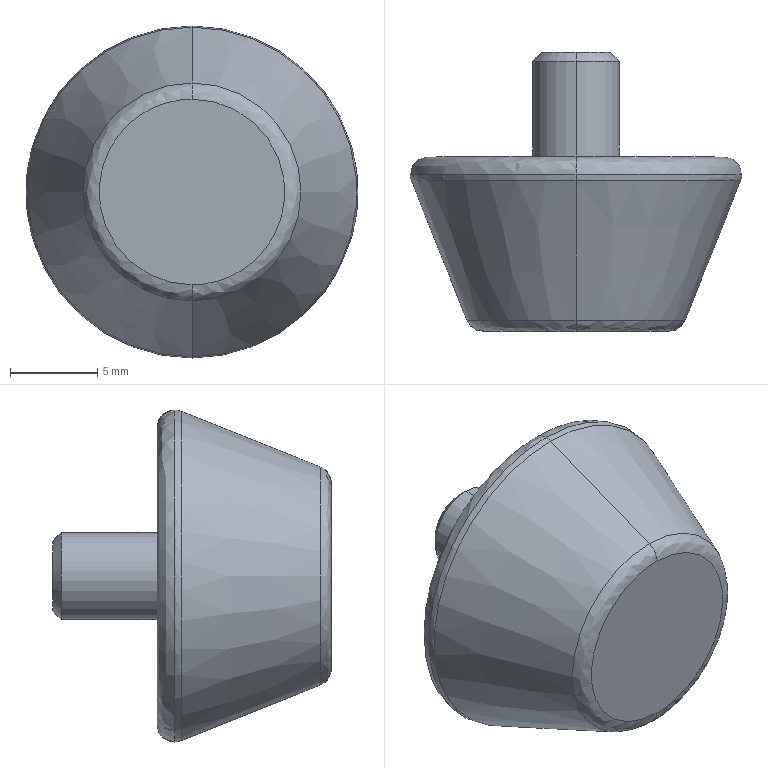Part | SolidWorks | features BaseBody 1 | 1 solid | 15 faces | box 19.046 x 16 x 19.046 mm | volume 2136 mm3 | spline 6 | cone 4 | plane 3 | cylinder 2 | commonest cylinder face diameters 5 x2
STEP:
#1=CARTESIAN_POINT('',(0.,9.,-9.523));
#2=VERTEX_POINT('',#1);
#3=CARTESIAN_POINT('',(0.,9.,9.523));
#4=VERTEX_POINT('',#3);
#5=CARTESIAN_POINT('',(0.,9.,0.));
#6=DIRECTION('',(0.,1.,0.));
#7=DIRECTION('',(0.,0.,1.));
#8=AXIS2_PLACEMENT_3D('',#5,#6,#7);
#9=CIRCLE('',#8,9.523);
#10=EDGE_CURVE('',#2,#4,#9,.T.);
#11=ORIENTED_EDGE('',*,*,#10,.F.);
#12=CARTESIAN_POINT('',(0.,8.629,-9.451));
#13=VERTEX_POINT('',#12);
#14=CARTESIAN_POINT('',(0.,9.,-8.523));
#15=DIRECTION('',(-1.,0.,0.));
#16=DIRECTION('',(0.,0.,-1.));
#17=AXIS2_PLACEMENT_3D('',#14,#15,#16);
#18=CIRCLE('',#17,1.);
#19=EDGE_CURVE('',#2,#13,#18,.T.);
#20=ORIENTED_EDGE('',*,*,#19,.T.);
#21=CARTESIAN_POINT('',(0.,8.629,9.451));
#22=VERTEX_POINT('',#21);
#23=CARTESIAN_POINT('',(0.,8.629,0.));
#24=DIRECTION('',(0.,-1.,0.));
#25=DIRECTION('',(0.,0.,1.));
#26=AXIS2_PLACEMENT_3D('',#23,#24,#25);
#27=CIRCLE('',#26,9.451);
#28=EDGE_CURVE('',#22,#13,#27,.T.);
#29=ORIENTED_EDGE('',*,*,#28,.F.);
#30=CARTESIAN_POINT('',(0.,9.,8.523));
#31=DIRECTION('',(1.,0.,0.));
#32=DIRECTION('',(0.,0.,1.));
#33=AXIS2_PLACEMENT_3D('',#30,#31,#32);
#34=CIRCLE('',#33,1.);
#35=EDGE_CURVE('',#4,#22,#34,.T.);
#36=ORIENTED_EDGE('',*,*,#35,.F.);
#37=EDGE_LOOP('',(#11,#20,#29,#36));
#38=FACE_OUTER_BOUND('',#37,.T.);
#39=CARTESIAN_POINT('',(0.,9.,-9.523));
#40=CARTESIAN_POINT('',(-19.046,9.,-9.523));
#41=CARTESIAN_POINT('',(-19.046,9.,9.523));
#42=CARTESIAN_POINT('',(0.,9.,9.523));
#43=CARTESIAN_POINT('',(0.,8.872,-9.523));
#44=CARTESIAN_POINT('',(-19.046,8.872,-9.523));
#45=CARTESIAN_POINT('',(-19.046,8.872,9.523));
#46=CARTESIAN_POINT('',(0.,8.872,9.523));
#47=CARTESIAN_POINT('',(0.,8.747,-9.499));
#48=CARTESIAN_POINT('',(-18.998,8.747,-9.499));
#49=CARTESIAN_POINT('',(-18.998,8.747,9.499));
#50=CARTESIAN_POINT('',(0.,8.747,9.499));
#51=CARTESIAN_POINT('',(0.,8.629,-9.451));
#52=CARTESIAN_POINT('',(-18.903,8.629,-9.451));
#53=CARTESIAN_POINT('',(-18.903,8.629,9.451));
#54=CARTESIAN_POINT('',(0.,8.629,9.451));
#55=(BOUNDED_SURFACE()B_SPLINE_SURFACE(3,3,((#39,#40,#41,#42),(#43,#44,#45,#46),(#47,#48,#49,#50),(#51,#52,#53,#54)),.UNSPECIFIED.,.F.,.F.,.F.)B_SPLINE_SURFACE_WITH_KNOTS((4,4),(4,4),(0.,1.),(0.,1.),.UNSPECIFIED.)GEOMETRIC_REPRESENTATION_ITEM()RATIONAL_B_SPLINE_SURFACE(((1.,0.3333,0.3333,1.),(0.988,0.3293,0.3293,0.988),(0.988,0.3293,0.3293,0.988),(1.,0.3333,0.3333,1.)))REPRESENTATION_ITEM('')SURFACE());
#56=ADVANCED_FACE('',(#38),#55,.T.);
#57=CARTESIAN_POINT('',(0.,0.6286,-6.251));
#58=VERTEX_POINT('',#57);
#59=CARTESIAN_POINT('',(0.,0.6286,6.251));
#60=VERTEX_POINT('',#59);
#61=CARTESIAN_POINT('',(0.,0.6286,0.));
#62=DIRECTION('',(0.,1.,0.));
#63=DIRECTION('',(0.,0.,1.));
#64=AXIS2_PLACEMENT_3D('',#61,#62,#63);
#65=CIRCLE('',#64,6.251);
#66=EDGE_CURVE('',#58,#60,#65,.T.);
#67=ORIENTED_EDGE('',*,*,#66,.F.);
#68=CARTESIAN_POINT('',(0.,0.,-5.323));
#69=VERTEX_POINT('',#68);
#70=CARTESIAN_POINT('',(0.,1.,-5.323));
#71=DIRECTION('',(-1.,0.,0.));
#72=DIRECTION('',(0.,0.,-1.));
#73=AXIS2_PLACEMENT_3D('',#70,#71,#72);
#74=CIRCLE('',#73,1.);
#75=EDGE_CURVE('',#58,#69,#74,.T.);
#76=ORIENTED_EDGE('',*,*,#75,.T.);
#77=CARTESIAN_POINT('',(0.,0.,5.323));
#78=VERTEX_POINT('',#77);
#79=CARTESIAN_POINT('',(0.,0.,-5.323));
#80=CARTESIAN_POINT('',(-10.646,0.,-5.323));
#81=CARTESIAN_POINT('',(-10.646,0.,5.323));
#82=CARTESIAN_POINT('',(0.,0.,5.323));
#83=(BOUNDED_CURVE()B_SPLINE_CURVE(3,(#79,#80,#81,#82),.UNSPECIFIED.,.F.,.F.)B_SPLINE_CURVE_WITH_KNOTS((4,4),(0.,1.),.UNSPECIFIED.)CURVE()GEOMETRIC_REPRESENTATION_ITEM()RATIONAL_B_SPLINE_CURVE((1.,0.3333,0.3333,1.))REPRESENTATION_ITEM(''));
#84=EDGE_CURVE('',#69,#78,#83,.T.);
#85=ORIENTED_EDGE('',*,*,#84,.T.);
#86=CARTESIAN_POINT('',(0.,1.,5.323));
#87=DIRECTION('',(1.,0.,0.));
#88=DIRECTION('',(0.,0.,1.));
#89=AXIS2_PLACEMENT_3D('',#86,#87,#88);
#90=CIRCLE('',#89,1.);
#91=EDGE_CURVE('',#60,#78,#90,.T.);
#92=ORIENTED_EDGE('',*,*,#91,.F.);
#93=EDGE_LOOP('',(#67,#76,#85,#92));
#94=FACE_OUTER_BOUND('',#93,.T.);
#95=CARTESIAN_POINT('',(0.,0.6286,-6.251));
#96=CARTESIAN_POINT('',(-12.503,0.6286,-6.251));
#97=CARTESIAN_POINT('',(-12.503,0.6286,6.251));
#98=CARTESIAN_POINT('',(0.,0.6286,6.251));
#99=CARTESIAN_POINT('',(0.,0.2367,-6.095));
#100=CARTESIAN_POINT('',(-12.189,0.2367,-6.095));
#101=CARTESIAN_POINT('',(-12.189,0.2367,6.095));
#102=CARTESIAN_POINT('',(0.,0.2367,6.095));
#103=CARTESIAN_POINT('',(0.,0.,-5.745));
#104=CARTESIAN_POINT('',(-11.49,0.,-5.745));
#105=CARTESIAN_POINT('',(-11.49,0.,5.745));
#106=CARTESIAN_POINT('',(0.,0.,5.745));
#107=CARTESIAN_POINT('',(0.,0.,-5.323));
#108=CARTESIAN_POINT('',(-10.646,0.,-5.323));
#109=CARTESIAN_POINT('',(-10.646,0.,5.323));
#110=CARTESIAN_POINT('',(0.,0.,5.323));
#111=(BOUNDED_SURFACE()B_SPLINE_SURFACE(3,3,((#95,#96,#97,#98),(#99,#100,#101,#102),(#103,#104,#105,#106),(#107,#108,#109,#110)),.UNSPECIFIED.,.F.,.F.,.F.)B_SPLINE_SURFACE_WITH_KNOTS((4,4),(4,4),(0.,1.),(0.,1.),.UNSPECIFIED.)GEOMETRIC_REPRESENTATION_ITEM()RATIONAL_B_SPLINE_SURFACE(((1.,0.3333,0.3333,1.),(0.8854,0.2951,0.2951,0.8854),(0.8854,0.2951,0.2951,0.8854),(1.,0.3333,0.3333,1.)))REPRESENTATION_ITEM('')SURFACE());
#112=ADVANCED_FACE('',(#94),#111,.T.);
#113=CARTESIAN_POINT('',(0.,10.,8.523));
#114=VERTEX_POINT('',#113);
#115=CARTESIAN_POINT('',(0.,10.,-8.523));
#116=VERTEX_POINT('',#115);
#117=CARTESIAN_POINT('',(0.,10.,8.523));
#118=CARTESIAN_POINT('',(-17.046,10.,8.523));
#119=CARTESIAN_POINT('',(-17.046,10.,-8.523));
#120=CARTESIAN_POINT('',(0.,10.,-8.523));
#121=(BOUNDED_CURVE()B_SPLINE_CURVE(3,(#117,#118,#119,#120),.UNSPECIFIED.,.F.,.F.)B_SPLINE_CURVE_WITH_KNOTS((4,4),(0.,1.),.UNSPECIFIED.)CURVE()GEOMETRIC_REPRESENTATION_ITEM()RATIONAL_B_SPLINE_CURVE((1.,0.3333,0.3333,1.))REPRESENTATION_ITEM(''));
#122=EDGE_CURVE('',#114,#116,#121,.T.);
#123=ORIENTED_EDGE('',*,*,#122,.T.);
#124=CARTESIAN_POINT('',(0.,9.,-8.523));
#125=DIRECTION('',(-1.,0.,0.));
#126=DIRECTION('',(0.,0.,-1.));
#127=AXIS2_PLACEMENT_3D('',#124,#125,#126);
#128=CIRCLE('',#127,1.);
#129=EDGE_CURVE('',#116,#2,#128,.T.);
#130=ORIENTED_EDGE('',*,*,#129,.T.);
#131=ORIENTED_EDGE('',*,*,#10,.T.);
#132=CARTESIAN_POINT('',(0.,9.,8.523));
#133=DIRECTION('',(1.,0.,0.));
#134=DIRECTION('',(0.,0.,1.));
#135=AXIS2_PLACEMENT_3D('',#132,#133,#134);
#136=CIRCLE('',#135,1.);
#137=EDGE_CURVE('',#114,#4,#136,.T.);
#138=ORIENTED_EDGE('',*,*,#137,.F.);
#139=EDGE_LOOP('',(#123,#130,#131,#138));
#140=FACE_OUTER_BOUND('',#139,.T.);
#141=CARTESIAN_POINT('',(0.,10.,-8.523));
#142=CARTESIAN_POINT('',(-17.046,10.,-8.523));
#143=CARTESIAN_POINT('',(-17.046,10.,8.523));
#144=CARTESIAN_POINT('',(0.,10.,8.523));
#145=CARTESIAN_POINT('',(0.,10.,-9.109));
#146=CARTESIAN_POINT('',(-18.218,10.,-9.109));
#147=CARTESIAN_POINT('',(-18.218,10.,9.109));
#148=CARTESIAN_POINT('',(0.,10.,9.109));
#149=CARTESIAN_POINT('',(0.,9.586,-9.523));
#150=CARTESIAN_POINT('',(-19.046,9.586,-9.523));
#151=CARTESIAN_POINT('',(-19.046,9.586,9.523));
#152=CARTESIAN_POINT('',(0.,9.586,9.523));
#153=CARTESIAN_POINT('',(0.,9.,-9.523));
#154=CARTESIAN_POINT('',(-19.046,9.,-9.523));
#155=CARTESIAN_POINT('',(-19.046,9.,9.523));
#156=CARTESIAN_POINT('',(0.,9.,9.523));
#157=(BOUNDED_SURFACE()B_SPLINE_SURFACE(3,3,((#141,#142,#143,#144),(#145,#146,#147,#148),(#149,#150,#151,#152),(#153,#154,#155,#156)),.UNSPECIFIED.,.F.,.F.,.F.)B_SPLINE_SURFACE_WITH_KNOTS((4,4),(4,4),(0.,1.),(0.,1.),.UNSPECIFIED.)GEOMETRIC_REPRESENTATION_ITEM()RATIONAL_B_SPLINE_SURFACE(((1.,0.3333,0.3333,1.),(0.8047,0.2682,0.2682,0.8047),(0.8047,0.2682,0.2682,0.8047),(1.,0.3333,0.3333,1.)))REPRESENTATION_ITEM('')SURFACE());
#158=ADVANCED_FACE('',(#140),#157,.T.);
#159=CARTESIAN_POINT('',(0.,0.6286,0.));
#160=DIRECTION('',(0.,1.,0.));
#161=DIRECTION('',(0.,0.,1.));
#162=AXIS2_PLACEMENT_3D('',#159,#160,#161);
#163=CIRCLE('',#162,6.251);
#164=EDGE_CURVE('',#60,#58,#163,.T.);
#165=ORIENTED_EDGE('',*,*,#164,.T.);
#166=CARTESIAN_POINT('',(0.,8.629,-9.451));
#167=DIRECTION('',(0.,0.9285,-0.3714));
#168=VECTOR('',#167,1000.);
#169=LINE('',#166,#168);
#170=EDGE_CURVE('',#58,#13,#169,.T.);
#171=ORIENTED_EDGE('',*,*,#170,.T.);
#172=CARTESIAN_POINT('',(0.,8.629,0.));
#173=DIRECTION('',(0.,-1.,0.));
#174=DIRECTION('',(0.,0.,1.));
#175=AXIS2_PLACEMENT_3D('',#172,#173,#174);
#176=CIRCLE('',#175,9.451);
#177=EDGE_CURVE('',#13,#22,#176,.T.);
#178=ORIENTED_EDGE('',*,*,#177,.T.);
#179=CARTESIAN_POINT('',(0.,8.629,9.451));
#180=DIRECTION('',(0.,0.9285,0.3714));
#181=VECTOR('',#180,1000.);
#182=LINE('',#179,#181);
#183=EDGE_CURVE('',#60,#22,#182,.T.);
#184=ORIENTED_EDGE('',*,*,#183,.F.);
#185=EDGE_LOOP('',(#165,#171,#178,#184));
#186=FACE_OUTER_BOUND('',#185,.T.);
#187=CARTESIAN_POINT('',(0.,8.629,0.));
#188=DIRECTION('',(0.,1.,0.));
#189=DIRECTION('',(0.,0.,1.));
#190=AXIS2_PLACEMENT_3D('',#187,#188,#189);
#191=CONICAL_SURFACE('',#190,9.451,0.3805);
#192=ADVANCED_FACE('',(#186),#191,.T.);
#193=ORIENTED_EDGE('',*,*,#129,.F.);
#194=CARTESIAN_POINT('',(0.,10.,-8.523));
#195=CARTESIAN_POINT('',(17.046,10.,-8.523));
#196=CARTESIAN_POINT('',(17.046,10.,8.523));
#197=CARTESIAN_POINT('',(0.,10.,8.523));
#198=(BOUNDED_CURVE()B_SPLINE_CURVE(3,(#194,#195,#196,#197),.UNSPECIFIED.,.F.,.F.)B_SPLINE_CURVE_WITH_KNOTS((4,4),(0.,1.),.UNSPECIFIED.)CURVE()GEOMETRIC_REPRESENTATION_ITEM()RATIONAL_B_SPLINE_CURVE((1.,0.3333,0.3333,1.))REPRESENTATION_ITEM(''));
#199=EDGE_CURVE('',#116,#114,#198,.T.);
#200=ORIENTED_EDGE('',*,*,#199,.T.);
#201=ORIENTED_EDGE('',*,*,#137,.T.);
#202=CARTESIAN_POINT('',(0.,9.,0.));
#203=DIRECTION('',(0.,1.,0.));
#204=DIRECTION('',(0.,0.,1.));
#205=AXIS2_PLACEMENT_3D('',#202,#203,#204);
#206=CIRCLE('',#205,9.523);
#207=EDGE_CURVE('',#4,#2,#206,.T.);
#208=ORIENTED_EDGE('',*,*,#207,.T.);
#209=EDGE_LOOP('',(#193,#200,#201,#208));
#210=FACE_OUTER_BOUND('',#209,.T.);
#211=CARTESIAN_POINT('',(0.,10.,8.523));
#212=CARTESIAN_POINT('',(17.046,10.,8.523));
#213=CARTESIAN_POINT('',(17.046,10.,-8.523));
#214=CARTESIAN_POINT('',(0.,10.,-8.523));
#215=CARTESIAN_POINT('',(0.,10.,9.109));
#216=CARTESIAN_POINT('',(18.218,10.,9.109));
#217=CARTESIAN_POINT('',(18.218,10.,-9.109));
#218=CARTESIAN_POINT('',(0.,10.,-9.109));
#219=CARTESIAN_POINT('',(0.,9.586,9.523));
#220=CARTESIAN_POINT('',(19.046,9.586,9.523));
#221=CARTESIAN_POINT('',(19.046,9.586,-9.523));
#222=CARTESIAN_POINT('',(0.,9.586,-9.523));
#223=CARTESIAN_POINT('',(0.,9.,9.523));
#224=CARTESIAN_POINT('',(19.046,9.,9.523));
#225=CARTESIAN_POINT('',(19.046,9.,-9.523));
#226=CARTESIAN_POINT('',(0.,9.,-9.523));
#227=(BOUNDED_SURFACE()B_SPLINE_SURFACE(3,3,((#211,#212,#213,#214),(#215,#216,#217,#218),(#219,#220,#221,#222),(#223,#224,#225,#226)),.UNSPECIFIED.,.F.,.F.,.F.)B_SPLINE_SURFACE_WITH_KNOTS((4,4),(4,4),(0.,1.),(0.,1.),.UNSPECIFIED.)GEOMETRIC_REPRESENTATION_ITEM()RATIONAL_B_SPLINE_SURFACE(((1.,0.3333,0.3333,1.),(0.8047,0.2682,0.2682,0.8047),(0.8047,0.2682,0.2682,0.8047),(1.,0.3333,0.3333,1.)))REPRESENTATION_ITEM('')SURFACE());
#228=ADVANCED_FACE('',(#210),#227,.T.);
#229=CARTESIAN_POINT('',(0.,10.,2.5));
#230=VERTEX_POINT('',#229);
#231=CARTESIAN_POINT('',(0.,10.,-2.5));
#232=VERTEX_POINT('',#231);
#233=CARTESIAN_POINT('',(0.,10.,0.));
#234=DIRECTION('',(0.,1.,0.));
#235=DIRECTION('',(0.,0.,1.));
#236=AXIS2_PLACEMENT_3D('',#233,#234,#235);
#237=CIRCLE('',#236,2.5);
#238=EDGE_CURVE('',#230,#232,#237,.T.);
#239=ORIENTED_EDGE('',*,*,#238,.T.);
#240=CARTESIAN_POINT('',(0.,15.5,-2.5));
#241=VERTEX_POINT('',#240);
#242=CARTESIAN_POINT('',(0.,16.,-2.5));
#243=DIRECTION('',(0.,1.,0.));
#244=VECTOR('',#243,1000.);
#245=LINE('',#242,#244);
#246=EDGE_CURVE('',#232,#241,#245,.T.);
#247=ORIENTED_EDGE('',*,*,#246,.T.);
#248=CARTESIAN_POINT('',(0.,15.5,2.5));
#249=VERTEX_POINT('',#248);
#250=CARTESIAN_POINT('',(0.,15.5,0.));
#251=DIRECTION('',(0.,-1.,0.));
#252=DIRECTION('',(0.,0.,1.));
#253=AXIS2_PLACEMENT_3D('',#250,#251,#252);
#254=CIRCLE('',#253,2.5);
#255=EDGE_CURVE('',#241,#249,#254,.T.);
#256=ORIENTED_EDGE('',*,*,#255,.T.);
#257=CARTESIAN_POINT('',(0.,16.,2.5));
#258=DIRECTION('',(0.,1.,0.));
#259=VECTOR('',#258,1000.);
#260=LINE('',#257,#259);
#261=EDGE_CURVE('',#230,#249,#260,.T.);
#262=ORIENTED_EDGE('',*,*,#261,.F.);
#263=EDGE_LOOP('',(#239,#247,#256,#262));
#264=FACE_OUTER_BOUND('',#263,.T.);
#265=CARTESIAN_POINT('',(0.,16.,0.));
#266=DIRECTION('',(0.,1.,0.));
#267=DIRECTION('',(0.,0.,1.));
#268=AXIS2_PLACEMENT_3D('',#265,#266,#267);
#269=CYLINDRICAL_SURFACE('',#268,2.5);
#270=ADVANCED_FACE('',(#264),#269,.T.);
#271=CARTESIAN_POINT('',(0.,16.,-2.));
#272=VERTEX_POINT('',#271);
#273=CARTESIAN_POINT('',(0.,16.,2.));
#274=VERTEX_POINT('',#273);
#275=CARTESIAN_POINT('',(0.,16.,0.));
#276=DIRECTION('',(0.,-1.,0.));
#277=DIRECTION('',(0.,0.,-1.));
#278=AXIS2_PLACEMENT_3D('',#275,#276,#277);
#279=CIRCLE('',#278,2.);
#280=EDGE_CURVE('',#272,#274,#279,.T.);
#281=ORIENTED_EDGE('',*,*,#280,.T.);
#282=CARTESIAN_POINT('',(0.,15.5,2.5));
#283=DIRECTION('',(0.,-0.7071,0.7071));
#284=VECTOR('',#283,1000.);
#285=LINE('',#282,#284);
#286=EDGE_CURVE('',#274,#249,#285,.T.);
#287=ORIENTED_EDGE('',*,*,#286,.T.);
#288=ORIENTED_EDGE('',*,*,#255,.F.);
#289=CARTESIAN_POINT('',(0.,15.5,-2.5));
#290=DIRECTION('',(0.,-0.7071,-0.7071));
#291=VECTOR('',#290,1000.);
#292=LINE('',#289,#291);
#293=EDGE_CURVE('',#272,#241,#292,.T.);
#294=ORIENTED_EDGE('',*,*,#293,.F.);
#295=EDGE_LOOP('',(#281,#287,#288,#294));
#296=FACE_OUTER_BOUND('',#295,.T.);
#297=CARTESIAN_POINT('',(0.,15.5,0.));
#298=DIRECTION('',(0.,-1.,0.));
#299=DIRECTION('',(0.,0.,-1.));
#300=AXIS2_PLACEMENT_3D('',#297,#298,#299);
#301=CONICAL_SURFACE('',#300,2.5,0.7854);
#302=ADVANCED_FACE('',(#296),#301,.T.);
#303=ORIENTED_EDGE('',*,*,#170,.F.);
#304=ORIENTED_EDGE('',*,*,#66,.T.);
#305=ORIENTED_EDGE('',*,*,#183,.T.);
#306=ORIENTED_EDGE('',*,*,#28,.T.);
#307=EDGE_LOOP('',(#303,#304,#305,#306));
#308=FACE_OUTER_BOUND('',#307,.T.);
#309=CARTESIAN_POINT('',(0.,8.629,0.));
#310=DIRECTION('',(0.,1.,0.));
#311=DIRECTION('',(0.,0.,1.));
#312=AXIS2_PLACEMENT_3D('',#309,#310,#311);
#313=CONICAL_SURFACE('',#312,9.451,0.3805);
#314=ADVANCED_FACE('',(#308),#313,.T.);
#315=ORIENTED_EDGE('',*,*,#19,.F.);
#316=ORIENTED_EDGE('',*,*,#207,.F.);
#317=ORIENTED_EDGE('',*,*,#35,.T.);
#318=ORIENTED_EDGE('',*,*,#177,.F.);
#319=EDGE_LOOP('',(#315,#316,#317,#318));
#320=FACE_OUTER_BOUND('',#319,.T.);
#321=CARTESIAN_POINT('',(0.,9.,9.523));
#322=CARTESIAN_POINT('',(19.046,9.,9.523));
#323=CARTESIAN_POINT('',(19.046,9.,-9.523));
#324=CARTESIAN_POINT('',(0.,9.,-9.523));
#325=CARTESIAN_POINT('',(0.,8.872,9.523));
#326=CARTESIAN_POINT('',(19.046,8.872,9.523));
#327=CARTESIAN_POINT('',(19.046,8.872,-9.523));
#328=CARTESIAN_POINT('',(0.,8.872,-9.523));
#329=CARTESIAN_POINT('',(0.,8.747,9.499));
#330=CARTESIAN_POINT('',(18.998,8.747,9.499));
#331=CARTESIAN_POINT('',(18.998,8.747,-9.499));
#332=CARTESIAN_POINT('',(0.,8.747,-9.499));
#333=CARTESIAN_POINT('',(0.,8.629,9.451));
#334=CARTESIAN_POINT('',(18.903,8.629,9.451));
#335=CARTESIAN_POINT('',(18.903,8.629,-9.451));
#336=CARTESIAN_POINT('',(0.,8.629,-9.451));
#337=(BOUNDED_SURFACE()B_SPLINE_SURFACE(3,3,((#321,#322,#323,#324),(#325,#326,#327,#328),(#329,#330,#331,#332),(#333,#334,#335,#336)),.UNSPECIFIED.,.F.,.F.,.F.)B_SPLINE_SURFACE_WITH_KNOTS((4,4),(4,4),(0.,1.),(0.,1.),.UNSPECIFIED.)GEOMETRIC_REPRESENTATION_ITEM()RATIONAL_B_SPLINE_SURFACE(((1.,0.3333,0.3333,1.),(0.988,0.3293,0.3293,0.988),(0.988,0.3293,0.3293,0.988),(1.,0.3333,0.3333,1.)))REPRESENTATION_ITEM('')SURFACE());
#338=ADVANCED_FACE('',(#320),#337,.T.);
#339=ORIENTED_EDGE('',*,*,#75,.F.);
#340=ORIENTED_EDGE('',*,*,#164,.F.);
#341=ORIENTED_EDGE('',*,*,#91,.T.);
#342=CARTESIAN_POINT('',(0.,0.,5.323));
#343=CARTESIAN_POINT('',(10.646,0.,5.323));
#344=CARTESIAN_POINT('',(10.646,0.,-5.323));
#345=CARTESIAN_POINT('',(0.,0.,-5.323));
#346=(BOUNDED_CURVE()B_SPLINE_CURVE(3,(#342,#343,#344,#345),.UNSPECIFIED.,.F.,.F.)B_SPLINE_CURVE_WITH_KNOTS((4,4),(0.,1.),.UNSPECIFIED.)CURVE()GEOMETRIC_REPRESENTATION_ITEM()RATIONAL_B_SPLINE_CURVE((1.,0.3333,0.3333,1.))REPRESENTATION_ITEM(''));
#347=EDGE_CURVE('',#78,#69,#346,.T.);
#348=ORIENTED_EDGE('',*,*,#347,.T.);
#349=EDGE_LOOP('',(#339,#340,#341,#348));
#350=FACE_OUTER_BOUND('',#349,.T.);
#351=CARTESIAN_POINT('',(0.,0.6286,6.251));
#352=CARTESIAN_POINT('',(12.503,0.6286,6.251));
#353=CARTESIAN_POINT('',(12.503,0.6286,-6.251));
#354=CARTESIAN_POINT('',(0.,0.6286,-6.251));
#355=CARTESIAN_POINT('',(0.,0.2367,6.095));
#356=CARTESIAN_POINT('',(12.189,0.2367,6.095));
#357=CARTESIAN_POINT('',(12.189,0.2367,-6.095));
#358=CARTESIAN_POINT('',(0.,0.2367,-6.095));
#359=CARTESIAN_POINT('',(0.,0.,5.745));
#360=CARTESIAN_POINT('',(11.49,0.,5.745));
#361=CARTESIAN_POINT('',(11.49,0.,-5.745));
#362=CARTESIAN_POINT('',(0.,0.,-5.745));
#363=CARTESIAN_POINT('',(0.,0.,5.323));
#364=CARTESIAN_POINT('',(10.646,0.,5.323));
#365=CARTESIAN_POINT('',(10.646,0.,-5.323));
#366=CARTESIAN_POINT('',(0.,0.,-5.323));
#367=(BOUNDED_SURFACE()B_SPLINE_SURFACE(3,3,((#351,#352,#353,#354),(#355,#356,#357,#358),(#359,#360,#361,#362),(#363,#364,#365,#366)),.UNSPECIFIED.,.F.,.F.,.F.)B_SPLINE_SURFACE_WITH_KNOTS((4,4),(4,4),(0.,1.),(0.,1.),.UNSPECIFIED.)GEOMETRIC_REPRESENTATION_ITEM()RATIONAL_B_SPLINE_SURFACE(((1.,0.3333,0.3333,1.),(0.8854,0.2951,0.2951,0.8854),(0.8854,0.2951,0.2951,0.8854),(1.,0.3333,0.3333,1.)))REPRESENTATION_ITEM('')SURFACE());
#368=ADVANCED_FACE('',(#350),#367,.T.);
#369=ORIENTED_EDGE('',*,*,#122,.F.);
#370=ORIENTED_EDGE('',*,*,#199,.F.);
#371=EDGE_LOOP('',(#369,#370));
#372=FACE_OUTER_BOUND('',#371,.T.);
#373=ORIENTED_EDGE('',*,*,#238,.F.);
#374=CARTESIAN_POINT('',(0.,10.,0.));
#375=DIRECTION('',(0.,1.,0.));
#376=DIRECTION('',(0.,0.,1.));
#377=AXIS2_PLACEMENT_3D('',#374,#375,#376);
#378=CIRCLE('',#377,2.5);
#379=EDGE_CURVE('',#232,#230,#378,.T.);
#380=ORIENTED_EDGE('',*,*,#379,.F.);
#381=EDGE_LOOP('',(#373,#380));
#382=FACE_BOUND('',#381,.T.);
#383=CARTESIAN_POINT('',(8.523,10.,0.));
#384=DIRECTION('',(0.,-1.,0.));
#385=DIRECTION('',(0.,0.,-1.));
#386=AXIS2_PLACEMENT_3D('',#383,#384,#385);
#387=PLANE('',#386);
#388=ADVANCED_FACE('',(#372,#382),#387,.F.);
#389=ORIENTED_EDGE('',*,*,#84,.F.);
#390=ORIENTED_EDGE('',*,*,#347,.F.);
#391=EDGE_LOOP('',(#389,#390));
#392=FACE_OUTER_BOUND('',#391,.T.);
#393=CARTESIAN_POINT('',(0.,0.,0.));
#394=DIRECTION('',(0.,1.,0.));
#395=DIRECTION('',(0.,0.,1.));
#396=AXIS2_PLACEMENT_3D('',#393,#394,#395);
#397=PLANE('',#396);
#398=ADVANCED_FACE('',(#392),#397,.F.);
#399=ORIENTED_EDGE('',*,*,#246,.F.);
#400=ORIENTED_EDGE('',*,*,#379,.T.);
#401=ORIENTED_EDGE('',*,*,#261,.T.);
#402=CARTESIAN_POINT('',(0.,15.5,0.));
#403=DIRECTION('',(0.,-1.,0.));
#404=DIRECTION('',(0.,0.,1.));
#405=AXIS2_PLACEMENT_3D('',#402,#403,#404);
#406=CIRCLE('',#405,2.5);
#407=EDGE_CURVE('',#249,#241,#406,.T.);
#408=ORIENTED_EDGE('',*,*,#407,.T.);
#409=EDGE_LOOP('',(#399,#400,#401,#408));
#410=FACE_OUTER_BOUND('',#409,.T.);
#411=CARTESIAN_POINT('',(0.,16.,0.));
#412=DIRECTION('',(0.,1.,0.));
#413=DIRECTION('',(0.,0.,1.));
#414=AXIS2_PLACEMENT_3D('',#411,#412,#413);
#415=CYLINDRICAL_SURFACE('',#414,2.5);
#416=ADVANCED_FACE('',(#410),#415,.T.);
#417=ORIENTED_EDGE('',*,*,#286,.F.);
#418=CARTESIAN_POINT('',(0.,16.,0.));
#419=DIRECTION('',(0.,-1.,0.));
#420=DIRECTION('',(0.,0.,-1.));
#421=AXIS2_PLACEMENT_3D('',#418,#419,#420);
#422=CIRCLE('',#421,2.);
#423=EDGE_CURVE('',#274,#272,#422,.T.);
#424=ORIENTED_EDGE('',*,*,#423,.T.);
#425=ORIENTED_EDGE('',*,*,#293,.T.);
#426=ORIENTED_EDGE('',*,*,#407,.F.);
#427=EDGE_LOOP('',(#417,#424,#425,#426));
#428=FACE_OUTER_BOUND('',#427,.T.);
#429=CARTESIAN_POINT('',(0.,15.5,0.));
#430=DIRECTION('',(0.,-1.,0.));
#431=DIRECTION('',(0.,0.,-1.));
#432=AXIS2_PLACEMENT_3D('',#429,#430,#431);
#433=CONICAL_SURFACE('',#432,2.5,0.7854);
#434=ADVANCED_FACE('',(#428),#433,.T.);
#435=ORIENTED_EDGE('',*,*,#280,.F.);
#436=ORIENTED_EDGE('',*,*,#423,.F.);
#437=EDGE_LOOP('',(#435,#436));
#438=FACE_OUTER_BOUND('',#437,.T.);
#439=CARTESIAN_POINT('',(2.5,16.,0.));
#440=DIRECTION('',(0.,-1.,0.));
#441=DIRECTION('',(0.,0.,-1.));
#442=AXIS2_PLACEMENT_3D('',#439,#440,#441);
#443=PLANE('',#442);
#444=ADVANCED_FACE('',(#438),#443,.F.);
#445=CLOSED_SHELL('',(#56,#112,#158,#192,#228,#270,#302,#314,#338,#368,#388,#398,#416,#434,#444));
#446=MANIFOLD_SOLID_BREP('',#445);
#447=CARTESIAN_POINT('',(0.,0.,0.));
#448=DIRECTION('',(0.,0.,1.));
#449=DIRECTION('',(1.,0.,0.));
#450=AXIS2_PLACEMENT_3D('',#447,#448,#449);
#451=(LENGTH_UNIT()NAMED_UNIT(*)SI_UNIT(.MILLI.,.METRE.));
#452=UNCERTAINTY_MEASURE_WITH_UNIT(LENGTH_MEASURE(0.00001),#451,'','');
#453=(NAMED_UNIT(*)PLANE_ANGLE_UNIT()SI_UNIT($,.RADIAN.));
#454=(NAMED_UNIT(*)SI_UNIT($,.STERADIAN.)SOLID_ANGLE_UNIT());
#455=(GEOMETRIC_REPRESENTATION_CONTEXT(3)GLOBAL_UNCERTAINTY_ASSIGNED_CONTEXT((#452))GLOBAL_UNIT_ASSIGNED_CONTEXT((#451,#453,#454))REPRESENTATION_CONTEXT('',''));
#456=ADVANCED_BREP_SHAPE_REPRESENTATION('',(#446,#450),#455);